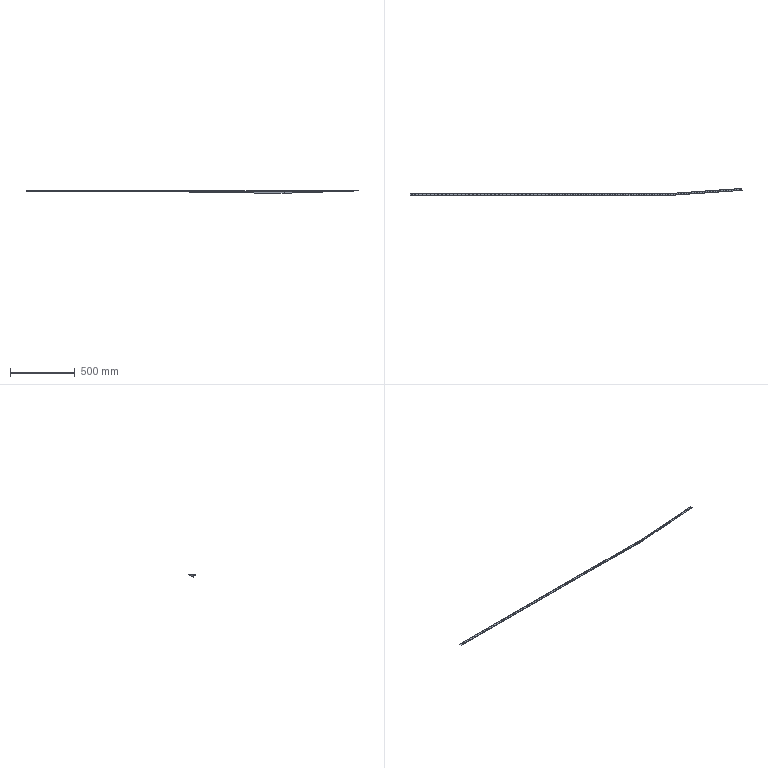Part | SolidWorks | features BaseBody 1 | 1 solid | 236 faces | box 2573 x 54.995 x 21.656 mm | volume 170781 mm3 | cylinder 220 | plane 16 | commonest cylinder face diameters 3.2 x220